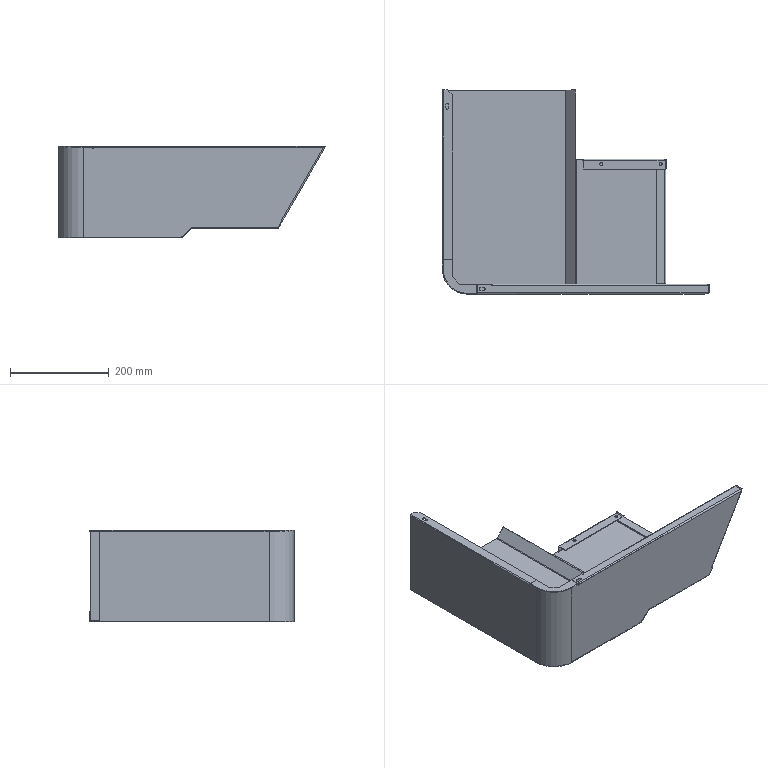Part | SolidWorks | 3 solids | 180 faces | box 540.3 x 413 x 185.75 mm | volume 547787 mm3 | plane 135 | cylinder 40 | spline 5 | commonest cylinder face diameters 4 x9 6.4 x8 1 x7 6 x4 2 x2 5 x2